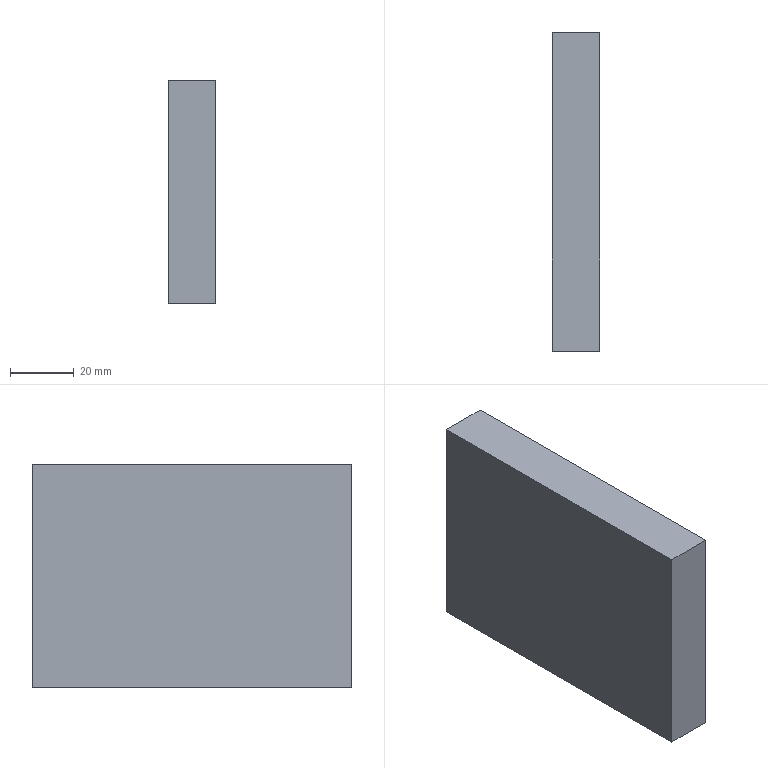Part | STEP file | Tube feed_id670_x_t | 1 solid | 6 faces | box 15 x 100 x 70 mm | volume 105000 mm3 | plane 6
STEP:
#1=CARTESIAN_POINT('',(0.,0.,0.));
#2=DIRECTION('',(0.,0.,1.));
#3=DIRECTION('',(1.,0.,0.));
#4=AXIS2_PLACEMENT_3D('',#1,#2,#3);
#5=CARTESIAN_POINT('',(126.,260.936,-50.15));
#6=VERTEX_POINT('',#5);
#7=CARTESIAN_POINT('',(126.,160.936,-50.15));
#8=VERTEX_POINT('',#7);
#9=CARTESIAN_POINT('',(126.,260.936,-50.15));
#10=DIRECTION('',(0.,-1.,0.));
#11=VECTOR('',#10,1.);
#12=LINE('',#9,#11);
#13=CARTESIAN_POINT('',(126.,260.936,19.85));
#14=DIRECTION('',(1.,0.,0.));
#15=DIRECTION('',(0.,0.,-1.));
#16=AXIS2_PLACEMENT_3D('',#13,#14,#15);
#17=PLANE('',#16);
#18=CARTESIAN_POINT('',(70.,0.));
#19=DIRECTION('',(0.,-1.));
#20=VECTOR('',#19,1.);
#21=LINE('',#18,#20);
#22=(GEOMETRIC_REPRESENTATION_CONTEXT(2)PARAMETRIC_REPRESENTATION_CONTEXT()REPRESENTATION_CONTEXT('',''));
#23=DEFINITIONAL_REPRESENTATION('',(#21),#22);
#24=PCURVE('',#17,#23);
#25=CARTESIAN_POINT('',(0.,0.,-50.15));
#26=DIRECTION('',(0.,0.,1.));
#27=DIRECTION('',(1.,0.,0.));
#28=AXIS2_PLACEMENT_3D('',#25,#26,#27);
#29=PLANE('',#28);
#30=CARTESIAN_POINT('',(126.,260.936));
#31=DIRECTION('',(0.,-1.));
#32=VECTOR('',#31,1.);
#33=LINE('',#30,#32);
#34=(GEOMETRIC_REPRESENTATION_CONTEXT(2)PARAMETRIC_REPRESENTATION_CONTEXT()REPRESENTATION_CONTEXT('',''));
#35=DEFINITIONAL_REPRESENTATION('',(#33),#34);
#36=PCURVE('',#29,#35);
#37=SURFACE_CURVE('',#12,(#24,#36),.PCURVE_S1.);
#38=EDGE_CURVE('',#6,#8,#37,.T.);
#39=ORIENTED_EDGE('',*,*,#38,.T.);
#40=CARTESIAN_POINT('',(126.,160.936,19.85));
#41=VERTEX_POINT('',#40);
#42=CARTESIAN_POINT('',(126.,160.936,19.85));
#43=DIRECTION('',(0.,0.,-1.));
#44=VECTOR('',#43,1.);
#45=LINE('',#42,#44);
#46=CARTESIAN_POINT('',(0.,-100.));
#47=DIRECTION('',(1.,0.));
#48=VECTOR('',#47,1.);
#49=LINE('',#46,#48);
#50=(GEOMETRIC_REPRESENTATION_CONTEXT(2)PARAMETRIC_REPRESENTATION_CONTEXT()REPRESENTATION_CONTEXT('',''));
#51=DEFINITIONAL_REPRESENTATION('',(#49),#50);
#52=PCURVE('',#17,#51);
#53=CARTESIAN_POINT('',(126.,160.936,19.85));
#54=DIRECTION('',(0.,1.,0.));
#55=DIRECTION('',(0.,0.,1.));
#56=AXIS2_PLACEMENT_3D('',#53,#54,#55);
#57=PLANE('',#56);
#58=CARTESIAN_POINT('',(0.,0.));
#59=DIRECTION('',(-1.,0.));
#60=VECTOR('',#59,1.);
#61=LINE('',#58,#60);
#62=(GEOMETRIC_REPRESENTATION_CONTEXT(2)PARAMETRIC_REPRESENTATION_CONTEXT()REPRESENTATION_CONTEXT('',''));
#63=DEFINITIONAL_REPRESENTATION('',(#61),#62);
#64=PCURVE('',#57,#63);
#65=SURFACE_CURVE('',#45,(#52,#64),.PCURVE_S1.);
#66=EDGE_CURVE('',#41,#8,#65,.T.);
#67=ORIENTED_EDGE('',*,*,#66,.F.);
#68=CARTESIAN_POINT('',(126.,260.936,19.85));
#69=VERTEX_POINT('',#68);
#70=CARTESIAN_POINT('',(126.,260.936,19.85));
#71=DIRECTION('',(0.,-1.,0.));
#72=VECTOR('',#71,1.);
#73=LINE('',#70,#72);
#74=CARTESIAN_POINT('',(0.,0.));
#75=DIRECTION('',(0.,-1.));
#76=VECTOR('',#75,1.);
#77=LINE('',#74,#76);
#78=(GEOMETRIC_REPRESENTATION_CONTEXT(2)PARAMETRIC_REPRESENTATION_CONTEXT()REPRESENTATION_CONTEXT('',''));
#79=DEFINITIONAL_REPRESENTATION('',(#77),#78);
#80=PCURVE('',#17,#79);
#81=CARTESIAN_POINT('',(0.,0.,19.85));
#82=DIRECTION('',(0.,0.,1.));
#83=DIRECTION('',(1.,0.,0.));
#84=AXIS2_PLACEMENT_3D('',#81,#82,#83);
#85=PLANE('',#84);
#86=CARTESIAN_POINT('',(126.,260.936));
#87=DIRECTION('',(0.,-1.));
#88=VECTOR('',#87,1.);
#89=LINE('',#86,#88);
#90=(GEOMETRIC_REPRESENTATION_CONTEXT(2)PARAMETRIC_REPRESENTATION_CONTEXT()REPRESENTATION_CONTEXT('',''));
#91=DEFINITIONAL_REPRESENTATION('',(#89),#90);
#92=PCURVE('',#85,#91);
#93=SURFACE_CURVE('',#73,(#80,#92),.PCURVE_S1.);
#94=EDGE_CURVE('',#69,#41,#93,.T.);
#95=ORIENTED_EDGE('',*,*,#94,.F.);
#96=CARTESIAN_POINT('',(126.,260.936,19.85));
#97=DIRECTION('',(0.,0.,-1.));
#98=VECTOR('',#97,1.);
#99=LINE('',#96,#98);
#100=CARTESIAN_POINT('',(0.,0.));
#101=DIRECTION('',(1.,0.));
#102=VECTOR('',#101,1.);
#103=LINE('',#100,#102);
#104=(GEOMETRIC_REPRESENTATION_CONTEXT(2)PARAMETRIC_REPRESENTATION_CONTEXT()REPRESENTATION_CONTEXT('',''));
#105=DEFINITIONAL_REPRESENTATION('',(#103),#104);
#106=PCURVE('',#17,#105);
#107=CARTESIAN_POINT('',(141.,260.936,19.85));
#108=DIRECTION('',(0.,-1.,0.));
#109=DIRECTION('',(0.,0.,-1.));
#110=AXIS2_PLACEMENT_3D('',#107,#108,#109);
#111=PLANE('',#110);
#112=CARTESIAN_POINT('',(0.,-15.));
#113=DIRECTION('',(1.,0.));
#114=VECTOR('',#113,1.);
#115=LINE('',#112,#114);
#116=(GEOMETRIC_REPRESENTATION_CONTEXT(2)PARAMETRIC_REPRESENTATION_CONTEXT()REPRESENTATION_CONTEXT('',''));
#117=DEFINITIONAL_REPRESENTATION('',(#115),#116);
#118=PCURVE('',#111,#117);
#119=SURFACE_CURVE('',#99,(#106,#118),.PCURVE_S1.);
#120=EDGE_CURVE('',#69,#6,#119,.T.);
#121=ORIENTED_EDGE('',*,*,#120,.T.);
#122=EDGE_LOOP('',(#39,#67,#95,#121));
#123=FACE_BOUND('',#122,.T.);
#124=ADVANCED_FACE('',(#123),#17,.F.);
#125=CARTESIAN_POINT('',(141.,160.936,-50.15));
#126=VERTEX_POINT('',#125);
#127=CARTESIAN_POINT('',(126.,160.936,-50.15));
#128=DIRECTION('',(1.,0.,0.));
#129=VECTOR('',#128,1.);
#130=LINE('',#127,#129);
#131=CARTESIAN_POINT('',(-70.,0.));
#132=DIRECTION('',(0.,1.));
#133=VECTOR('',#132,1.);
#134=LINE('',#131,#133);
#135=(GEOMETRIC_REPRESENTATION_CONTEXT(2)PARAMETRIC_REPRESENTATION_CONTEXT()REPRESENTATION_CONTEXT('',''));
#136=DEFINITIONAL_REPRESENTATION('',(#134),#135);
#137=PCURVE('',#57,#136);
#138=CARTESIAN_POINT('',(126.,160.936));
#139=DIRECTION('',(1.,0.));
#140=VECTOR('',#139,1.);
#141=LINE('',#138,#140);
#142=(GEOMETRIC_REPRESENTATION_CONTEXT(2)PARAMETRIC_REPRESENTATION_CONTEXT()REPRESENTATION_CONTEXT('',''));
#143=DEFINITIONAL_REPRESENTATION('',(#141),#142);
#144=PCURVE('',#29,#143);
#145=SURFACE_CURVE('',#130,(#137,#144),.PCURVE_S1.);
#146=EDGE_CURVE('',#8,#126,#145,.T.);
#147=ORIENTED_EDGE('',*,*,#146,.T.);
#148=CARTESIAN_POINT('',(141.,160.936,19.85));
#149=VERTEX_POINT('',#148);
#150=CARTESIAN_POINT('',(141.,160.936,19.85));
#151=DIRECTION('',(0.,0.,-1.));
#152=VECTOR('',#151,1.);
#153=LINE('',#150,#152);
#154=CARTESIAN_POINT('',(0.,15.));
#155=DIRECTION('',(-1.,0.));
#156=VECTOR('',#155,1.);
#157=LINE('',#154,#156);
#158=(GEOMETRIC_REPRESENTATION_CONTEXT(2)PARAMETRIC_REPRESENTATION_CONTEXT()REPRESENTATION_CONTEXT('',''));
#159=DEFINITIONAL_REPRESENTATION('',(#157),#158);
#160=PCURVE('',#57,#159);
#161=CARTESIAN_POINT('',(141.,160.936,19.85));
#162=DIRECTION('',(-1.,0.,0.));
#163=DIRECTION('',(0.,-1.,0.));
#164=AXIS2_PLACEMENT_3D('',#161,#162,#163);
#165=PLANE('',#164);
#166=CARTESIAN_POINT('',(0.,0.));
#167=DIRECTION('',(0.,-1.));
#168=VECTOR('',#167,1.);
#169=LINE('',#166,#168);
#170=(GEOMETRIC_REPRESENTATION_CONTEXT(2)PARAMETRIC_REPRESENTATION_CONTEXT()REPRESENTATION_CONTEXT('',''));
#171=DEFINITIONAL_REPRESENTATION('',(#169),#170);
#172=PCURVE('',#165,#171);
#173=SURFACE_CURVE('',#153,(#160,#172),.PCURVE_S1.);
#174=EDGE_CURVE('',#149,#126,#173,.T.);
#175=ORIENTED_EDGE('',*,*,#174,.F.);
#176=CARTESIAN_POINT('',(126.,160.936,19.85));
#177=DIRECTION('',(1.,0.,0.));
#178=VECTOR('',#177,1.);
#179=LINE('',#176,#178);
#180=CARTESIAN_POINT('',(0.,0.));
#181=DIRECTION('',(0.,1.));
#182=VECTOR('',#181,1.);
#183=LINE('',#180,#182);
#184=(GEOMETRIC_REPRESENTATION_CONTEXT(2)PARAMETRIC_REPRESENTATION_CONTEXT()REPRESENTATION_CONTEXT('',''));
#185=DEFINITIONAL_REPRESENTATION('',(#183),#184);
#186=PCURVE('',#57,#185);
#187=CARTESIAN_POINT('',(126.,160.936));
#188=DIRECTION('',(1.,0.));
#189=VECTOR('',#188,1.);
#190=LINE('',#187,#189);
#191=(GEOMETRIC_REPRESENTATION_CONTEXT(2)PARAMETRIC_REPRESENTATION_CONTEXT()REPRESENTATION_CONTEXT('',''));
#192=DEFINITIONAL_REPRESENTATION('',(#190),#191);
#193=PCURVE('',#85,#192);
#194=SURFACE_CURVE('',#179,(#186,#193),.PCURVE_S1.);
#195=EDGE_CURVE('',#41,#149,#194,.T.);
#196=ORIENTED_EDGE('',*,*,#195,.F.);
#197=ORIENTED_EDGE('',*,*,#66,.T.);
#198=EDGE_LOOP('',(#147,#175,#196,#197));
#199=FACE_BOUND('',#198,.T.);
#200=ADVANCED_FACE('',(#199),#57,.F.);
#201=CARTESIAN_POINT('',(141.,260.936,-50.15));
#202=VERTEX_POINT('',#201);
#203=CARTESIAN_POINT('',(141.,160.936,-50.15));
#204=DIRECTION('',(0.,1.,0.));
#205=VECTOR('',#204,1.);
#206=LINE('',#203,#205);
#207=CARTESIAN_POINT('',(0.,-70.));
#208=DIRECTION('',(-1.,0.));
#209=VECTOR('',#208,1.);
#210=LINE('',#207,#209);
#211=(GEOMETRIC_REPRESENTATION_CONTEXT(2)PARAMETRIC_REPRESENTATION_CONTEXT()REPRESENTATION_CONTEXT('',''));
#212=DEFINITIONAL_REPRESENTATION('',(#210),#211);
#213=PCURVE('',#165,#212);
#214=CARTESIAN_POINT('',(141.,160.936));
#215=DIRECTION('',(0.,1.));
#216=VECTOR('',#215,1.);
#217=LINE('',#214,#216);
#218=(GEOMETRIC_REPRESENTATION_CONTEXT(2)PARAMETRIC_REPRESENTATION_CONTEXT()REPRESENTATION_CONTEXT('',''));
#219=DEFINITIONAL_REPRESENTATION('',(#217),#218);
#220=PCURVE('',#29,#219);
#221=SURFACE_CURVE('',#206,(#213,#220),.PCURVE_S1.);
#222=EDGE_CURVE('',#126,#202,#221,.T.);
#223=ORIENTED_EDGE('',*,*,#222,.T.);
#224=CARTESIAN_POINT('',(141.,260.936,19.85));
#225=VERTEX_POINT('',#224);
#226=CARTESIAN_POINT('',(141.,260.936,19.85));
#227=DIRECTION('',(0.,0.,-1.));
#228=VECTOR('',#227,1.);
#229=LINE('',#226,#228);
#230=CARTESIAN_POINT('',(-100.,0.));
#231=DIRECTION('',(0.,-1.));
#232=VECTOR('',#231,1.);
#233=LINE('',#230,#232);
#234=(GEOMETRIC_REPRESENTATION_CONTEXT(2)PARAMETRIC_REPRESENTATION_CONTEXT()REPRESENTATION_CONTEXT('',''));
#235=DEFINITIONAL_REPRESENTATION('',(#233),#234);
#236=PCURVE('',#165,#235);
#237=CARTESIAN_POINT('',(0.,0.));
#238=DIRECTION('',(1.,0.));
#239=VECTOR('',#238,1.);
#240=LINE('',#237,#239);
#241=(GEOMETRIC_REPRESENTATION_CONTEXT(2)PARAMETRIC_REPRESENTATION_CONTEXT()REPRESENTATION_CONTEXT('',''));
#242=DEFINITIONAL_REPRESENTATION('',(#240),#241);
#243=PCURVE('',#111,#242);
#244=SURFACE_CURVE('',#229,(#236,#243),.PCURVE_S1.);
#245=EDGE_CURVE('',#225,#202,#244,.T.);
#246=ORIENTED_EDGE('',*,*,#245,.F.);
#247=CARTESIAN_POINT('',(141.,160.936,19.85));
#248=DIRECTION('',(0.,1.,0.));
#249=VECTOR('',#248,1.);
#250=LINE('',#247,#249);
#251=CARTESIAN_POINT('',(0.,0.));
#252=DIRECTION('',(-1.,0.));
#253=VECTOR('',#252,1.);
#254=LINE('',#251,#253);
#255=(GEOMETRIC_REPRESENTATION_CONTEXT(2)PARAMETRIC_REPRESENTATION_CONTEXT()REPRESENTATION_CONTEXT('',''));
#256=DEFINITIONAL_REPRESENTATION('',(#254),#255);
#257=PCURVE('',#165,#256);
#258=CARTESIAN_POINT('',(141.,160.936));
#259=DIRECTION('',(0.,1.));
#260=VECTOR('',#259,1.);
#261=LINE('',#258,#260);
#262=(GEOMETRIC_REPRESENTATION_CONTEXT(2)PARAMETRIC_REPRESENTATION_CONTEXT()REPRESENTATION_CONTEXT('',''));
#263=DEFINITIONAL_REPRESENTATION('',(#261),#262);
#264=PCURVE('',#85,#263);
#265=SURFACE_CURVE('',#250,(#257,#264),.PCURVE_S1.);
#266=EDGE_CURVE('',#149,#225,#265,.T.);
#267=ORIENTED_EDGE('',*,*,#266,.F.);
#268=ORIENTED_EDGE('',*,*,#174,.T.);
#269=EDGE_LOOP('',(#223,#246,#267,#268));
#270=FACE_BOUND('',#269,.T.);
#271=ADVANCED_FACE('',(#270),#165,.F.);
#272=CARTESIAN_POINT('',(141.,260.936,-50.15));
#273=DIRECTION('',(-1.,0.,0.));
#274=VECTOR('',#273,1.);
#275=LINE('',#272,#274);
#276=CARTESIAN_POINT('',(70.,0.));
#277=DIRECTION('',(0.,-1.));
#278=VECTOR('',#277,1.);
#279=LINE('',#276,#278);
#280=(GEOMETRIC_REPRESENTATION_CONTEXT(2)PARAMETRIC_REPRESENTATION_CONTEXT()REPRESENTATION_CONTEXT('',''));
#281=DEFINITIONAL_REPRESENTATION('',(#279),#280);
#282=PCURVE('',#111,#281);
#283=CARTESIAN_POINT('',(141.,260.936));
#284=DIRECTION('',(-1.,0.));
#285=VECTOR('',#284,1.);
#286=LINE('',#283,#285);
#287=(GEOMETRIC_REPRESENTATION_CONTEXT(2)PARAMETRIC_REPRESENTATION_CONTEXT()REPRESENTATION_CONTEXT('',''));
#288=DEFINITIONAL_REPRESENTATION('',(#286),#287);
#289=PCURVE('',#29,#288);
#290=SURFACE_CURVE('',#275,(#282,#289),.PCURVE_S1.);
#291=EDGE_CURVE('',#202,#6,#290,.T.);
#292=ORIENTED_EDGE('',*,*,#291,.T.);
#293=ORIENTED_EDGE('',*,*,#120,.F.);
#294=CARTESIAN_POINT('',(141.,260.936,19.85));
#295=DIRECTION('',(-1.,0.,0.));
#296=VECTOR('',#295,1.);
#297=LINE('',#294,#296);
#298=CARTESIAN_POINT('',(0.,0.));
#299=DIRECTION('',(0.,-1.));
#300=VECTOR('',#299,1.);
#301=LINE('',#298,#300);
#302=(GEOMETRIC_REPRESENTATION_CONTEXT(2)PARAMETRIC_REPRESENTATION_CONTEXT()REPRESENTATION_CONTEXT('',''));
#303=DEFINITIONAL_REPRESENTATION('',(#301),#302);
#304=PCURVE('',#111,#303);
#305=CARTESIAN_POINT('',(141.,260.936));
#306=DIRECTION('',(-1.,0.));
#307=VECTOR('',#306,1.);
#308=LINE('',#305,#307);
#309=(GEOMETRIC_REPRESENTATION_CONTEXT(2)PARAMETRIC_REPRESENTATION_CONTEXT()REPRESENTATION_CONTEXT('',''));
#310=DEFINITIONAL_REPRESENTATION('',(#308),#309);
#311=PCURVE('',#85,#310);
#312=SURFACE_CURVE('',#297,(#304,#311),.PCURVE_S1.);
#313=EDGE_CURVE('',#225,#69,#312,.T.);
#314=ORIENTED_EDGE('',*,*,#313,.F.);
#315=ORIENTED_EDGE('',*,*,#245,.T.);
#316=EDGE_LOOP('',(#292,#293,#314,#315));
#317=FACE_BOUND('',#316,.T.);
#318=ADVANCED_FACE('',(#317),#111,.F.);
#319=ORIENTED_EDGE('',*,*,#94,.T.);
#320=ORIENTED_EDGE('',*,*,#195,.T.);
#321=ORIENTED_EDGE('',*,*,#266,.T.);
#322=ORIENTED_EDGE('',*,*,#313,.T.);
#323=EDGE_LOOP('',(#319,#320,#321,#322));
#324=FACE_BOUND('',#323,.T.);
#325=ADVANCED_FACE('',(#324),#85,.T.);
#326=ORIENTED_EDGE('',*,*,#38,.F.);
#327=ORIENTED_EDGE('',*,*,#291,.F.);
#328=ORIENTED_EDGE('',*,*,#222,.F.);
#329=ORIENTED_EDGE('',*,*,#146,.F.);
#330=EDGE_LOOP('',(#326,#327,#328,#329));
#331=FACE_BOUND('',#330,.T.);
#332=ADVANCED_FACE('',(#331),#29,.F.);
#333=CLOSED_SHELL('',(#124,#200,#271,#318,#325,#332));
#334=MANIFOLD_SOLID_BREP('',#333);
#335=(LENGTH_UNIT()NAMED_UNIT(*)SI_UNIT(.MILLI.,.METRE.));
#336=UNCERTAINTY_MEASURE_WITH_UNIT(LENGTH_MEASURE(0.0000001),#335,'','');
#337=(NAMED_UNIT(*)PLANE_ANGLE_UNIT()SI_UNIT($,.RADIAN.));
#338=(NAMED_UNIT(*)SI_UNIT($,.STERADIAN.)SOLID_ANGLE_UNIT());
#339=(GEOMETRIC_REPRESENTATION_CONTEXT(3)GLOBAL_UNCERTAINTY_ASSIGNED_CONTEXT((#336))GLOBAL_UNIT_ASSIGNED_CONTEXT((#335,#337,#338))REPRESENTATION_CONTEXT('',''));
#340=ADVANCED_BREP_SHAPE_REPRESENTATION('',(#4,#334),#339);